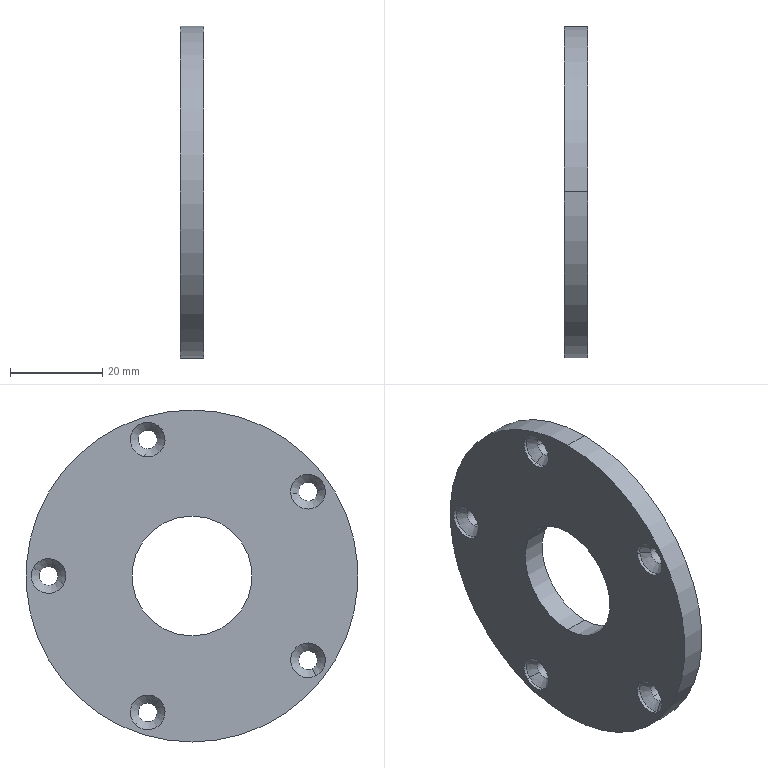Part | STEP file | Completa.sldasm-Part-111_Valor predeterminado | 1 solid | 36 faces | box 5.18 x 71.978 x 71.978 mm | volume 17752 mm3 | cylinder 24 | cone 10 | plane 2 | commonest cylinder face diameters 4.117 x10 7.53 x10 26 x2 71.978 x2